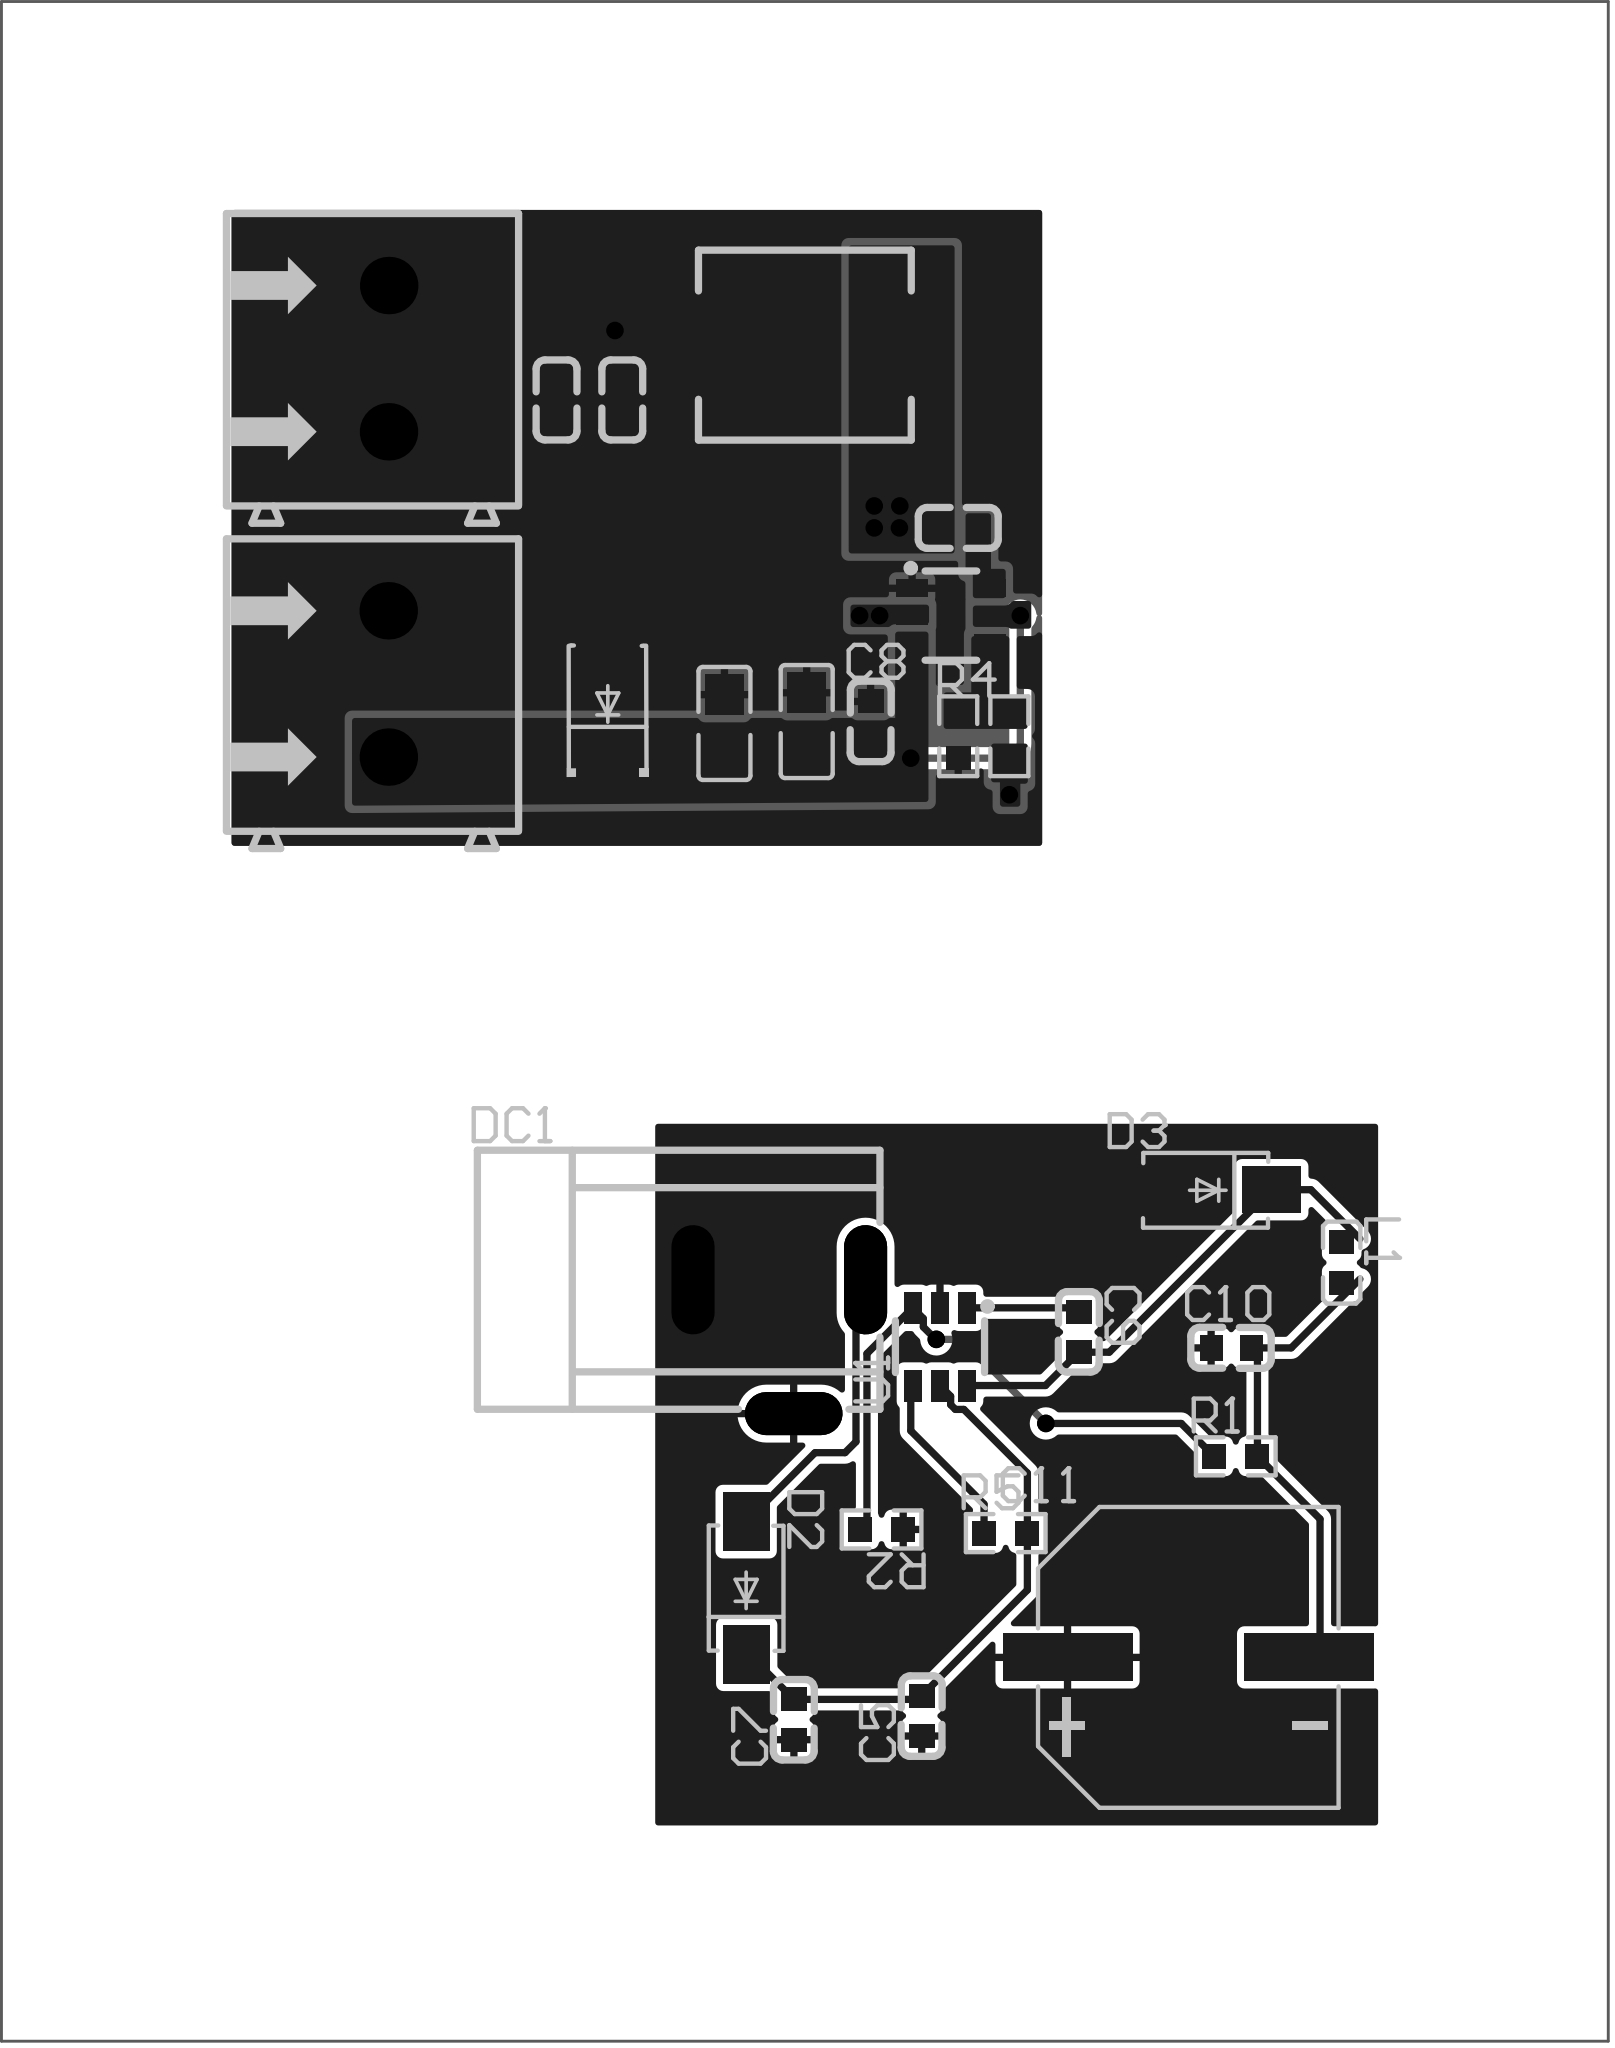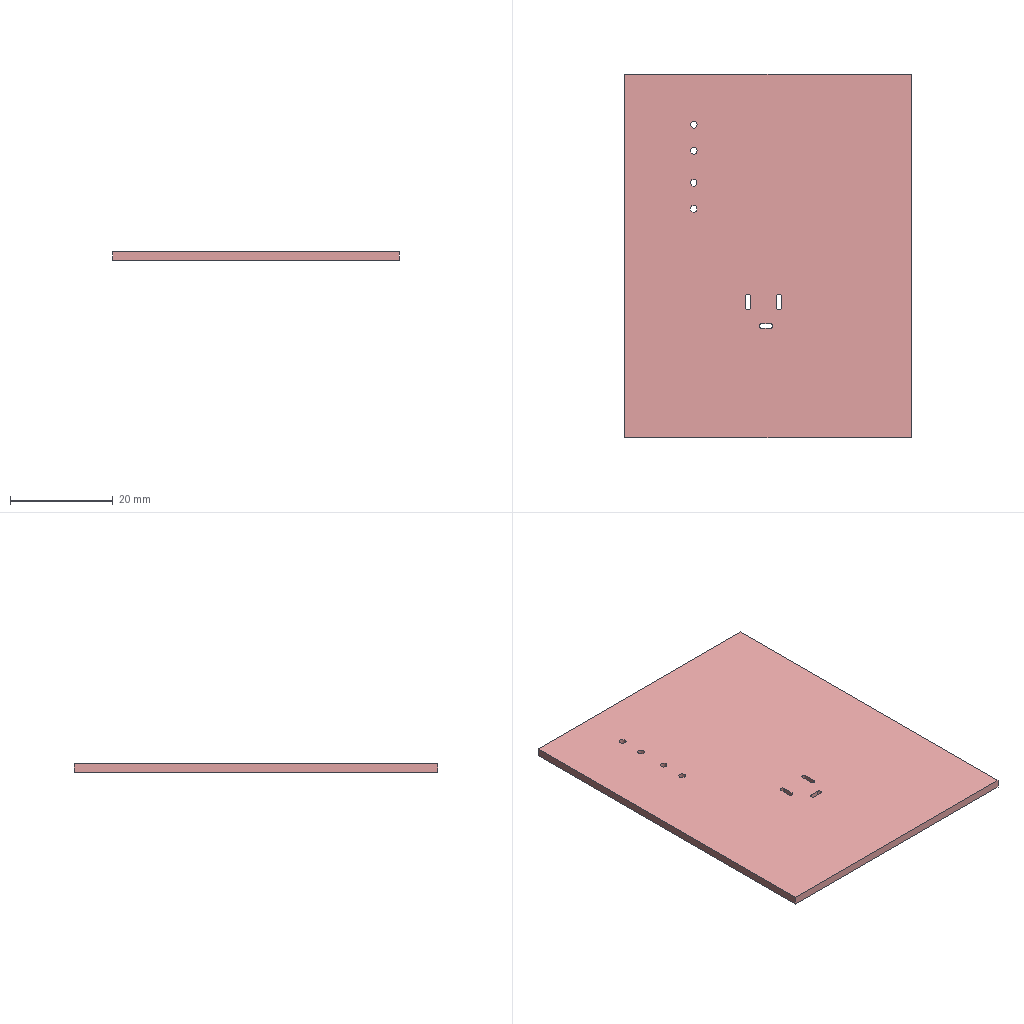Circuit board layout | Altium Designer | box 55.9 x 70.9 x 1.6 mm
Layer stack:
# Altium Designer layer stack of  (unit mm; dielectric type: 0 none, 1 core, 2 prepreg, 3 surface material)
index,name,kind,layer,copper_thickness_mm,dielectric_type,dielectric_thickness_mm,dielectric_material,dielectric_constant
0,Top Paste Mask Layer,other,,,,,,
1,Top Silkscreen Layer,other,,,,,,
2,Top Solder Mask Layer,dielectric,,,3,0.01,,3.3
3,Top Layer,copper,Top Layer,0.035,,,,
4,DIELECTRIC1,dielectric,,,3,1.51,FR4,4.5
5,Bottom Layer,copper,Bottom Layer,0.035,,,,
6,Bottom Solder Mask Layer,dielectric,,,3,0.01,,3.3
7,Bottom Silkscreen Layer,other,,,,,,
8,Bottom Paste Mask Layer,other,,,,,,
# drill layer pairs: low layer,high layer
drill_pair,Top Layer,Bottom Layer
Part placement:
Designator,Comment,Layer,Footprint,Center-X(mm),Center-Y(mm),Rotation
C8,100nF,TopLayer,C0603,100.076,115.697,270
R3,53.6kΩ,TopLayer,R0603,104.902,115.189,270
R4,10kΩ,TopLayer,R0603,103.124,115.189,90
C2,100nF,TopLayer,C0603,103.124,122.428,0
C3,22uF,TopLayer,C0603,89.154,126.873,90
U3,3.3uH,TopLayer,IND-SMD_L7.4-W6.6,97.79,128.778,180
C1,10uF,TopLayer,C0805,94.993,115.633,270
P1,WJ500V-5.08-2P,TopLayer,CONN-TH_2P-P5.00_WJ500V-5.08-2P,83.303,117.007,90
P2,WJ500V-5.08-2P,TopLayer,CONN-TH_2P-P5.00_WJ500V-5.08-2P,83.314,128.307,90
U2,TPS563201DDCR,TopLayer,SOT-23-6_L2.9-W1.6-P0.95-LS2.8-BR,102.87,119.38,180
C4,10uF,TopLayer,C0805,97.853,115.7,270
C6,22uF,TopLayer,C0603,91.44,126.873,90
D1,SMAJ12A,TopLayer,DO-214AC_L4.3-W2.7-LS5.0-RD,90.932,116.205,90
C5,10uF,TopLayer,C0603,101.854,81.153,90
C7,100nF,TopLayer,C0603,97.409,81.026,90
C9,100nF,TopLayer,C0603,107.315,94.488,270
C10,100nF,TopLayer,C0603,112.618,93.938,0
C11,220uF,TopLayer,CAP-SMD_BD10.0-L10.3-W10.3-LS11.7-FD,111.125,83.185,0
D2,SS14,TopLayer,SMA_L4.3-W2.6-LS5.0-FD,95.758,85.598,270
D3,SS14,TopLayer,SMA_L4.3-W2.6-LS5.0-FD,111.719,99.424,0
DC1,DC-005-A200,TopLayer,DC-IN-TH_DC-005-A200,96.902,93.981,0
L1,4.7uH,TopLayer,L0603,116.459,96.901,270
R1,49.9kΩ,TopLayer,R0603,112.776,90.17,0
R2,9.53kΩ,TopLayer,R0603,100.457,87.63,180
R5,100kΩ,TopLayer,R0603,104.775,87.503,0
U1,MP2359DT-LF-Z,TopLayer,SOT-23-6_L2.9-W1.6-P0.95-LS2.8-BR,102.489,93.98,90
Pad and via stacks:
# Altium Designer via and pad stacks of  (unit mm). Each distinct definition once, with the count of objects using it.
# via: kind,start_layer,end_layer,hole_mm,diameter_mm,mode(0 simple;1 top-mid-bottom;2 full stack),diameter_per_layer,count,example_net
# pad: kind,layer,hole_mm,hole_type(0 round;1 square;2 slot),plating,top_size,top_shape(1 round;2 rect;3 octagon;9 rounded rect),mid_size,bottom_size,mode,footprint,size_per_layer,count,example
pad,Top Layer,0,0,plated,0.8x0.9,2,0.8x0.9,0.8x0.9,0,C0603,,16,C8.2
pad,Top Layer,0,0,plated,0.8065x0.864,2,0.8065x0.864,0.8065x0.864,0,R0603,,10,R3.2
pad,Top Layer,0,0,plated,2.5x3.3,2,2.5x3.3,2.5x3.3,0,IND-SMD_L7.4-W6.6,,2,U3.1
pad,Top Layer,0,0,plated,1.41x1.35,2,1.41x1.35,1.41x1.35,0,C0805,,4,C1.2
pad,Top Layer,0,0,plated,1.1x0.6,2,1.1x0.6,1.1x0.6,0,SOT-23-6_L2.9-W1.6-P0.95-LS2.8-BR,,12,U2.3
pad,Top Layer,0,0,plated,2.07x2.06,2,2.07x2.06,2.07x2.06,0,DO-214AC_L4.3-W2.7-LS5.0-RD,,2,D1.1
pad,Top Layer,0,0,plated,4.5x1.65,2,4.5x1.65,4.5x1.65,0,CAP-SMD_BD10.0-L10.3-W10.3-LS11.7-FD,,2,C11.2
pad,Top Layer,0,0,plated,2.046x1.62,2,2.046x1.62,2.046x1.62,0,SMA_L4.3-W2.6-LS5.0-FD,,4,D2.1
pad,Top Layer,0,0,plated,0.8x0.864,2,0.8x0.864,0.8x0.864,0,L0603,,2,L1.1
pad,Multi-Layer,1.3,0,plated,2x2,1,2x2,2x2,0,CONN-TH_2P-P5.00_WJ500V-5.08-2P,,4,P1.2
pad,Multi-Layer,0.9,2,plated,1.5x3.8,1,1.5x3.8,1.5x3.8,0,DC-IN-TH_DC-005-A200,,2,DC1.1
pad,Multi-Layer,0.9,2,plated,1.5x3.4,1,1.5x3.4,1.5x3.4,0,DC-IN-TH_DC-005-A200,,1,DC1.3
via,Top Layer,Bottom Layer,0.3048,0.61,0,,12,$1N3805
Copper pours:
name,layer,net,type(0 solid;1 hatched;2 none)
Top Layer-$1N3805,Top Layer,$1N3805,0
Top Layer-$1N3766,Top Layer,$1N3766,0
Top Layer-+12V,Top Layer,+12V,0
Top Layer-$1N3805 1,Top Layer,$1N3805,0
Top Layer-+5V,Top Layer,+5V,0
Top Layer-$1N3448,Top Layer,$1N3448,0
Top Layer-+12V 1,Top Layer,+12V,0
Top Layer-GND,Top Layer,GND,0
Top Layer-+5V 1,Top Layer,+5V,0
Top Layer-GND 1,Top Layer,GND,0
Bottom Layer-$1N3805,Bottom Layer,$1N3805,0
Bottom Layer-GND,Bottom Layer,GND,0
Design rules, without the lines most boards share:
# Altium Designer design rules of  (exported by Altium Designer, unit mm)
# columns: name | kind | enabled | priority | scope1 | scope2 | descriptor | typed fields (field=value)
Copper_copperRegion1 | 0 | disabled | 4 | All | All | Clearance Constraint (Gap=5.984mil) (Disabled)(All),(All) | gap=0.152
Copper_copperRegion1_1 | 63 | disabled | 4 | All | All | Board Clearance Constraint (Gap=0mil) (Disabled)(All) |
copperThickness1oz | 0 | enabled | 5 | All | All | Clearance Constraint (Gap=5.984mil) (All),(All) | gap=0.152
copperThickness1oz_1 | 63 | enabled | 5 | All | All | Board Clearance Constraint (Gap=0mil) (All) |
copperRegion1 | 20 | disabled | 1 | All | All | Polygon Connect Rule(Direct Connect )(Conductor Width=10mil) (Relief Angle=90 Angle) (Entries=4) (Air Gap Width=10mil) (Disabled)(All),(All) | connect_style(0=relief,1=direct,2=none)=1 relief_conductor_width=0.254 relief_entries=4
copperRegion | 20 | enabled | 2 | All | All | Polygon Connect Rule(Relief Connect )(Conductor Width=10mil) (Relief Angle=90 Angle) (Entries=4) (Air Gap Width=10mil) (All),(All) | connect_style(0=relief,1=direct,2=none)=0 relief_conductor_width=0.254 relief_entries=4
solderMaskExpansion | 13 | enabled | 2 | All | All | Solder Mask Expansion (Expansion =2.008mil) (All) | expansion=0.051